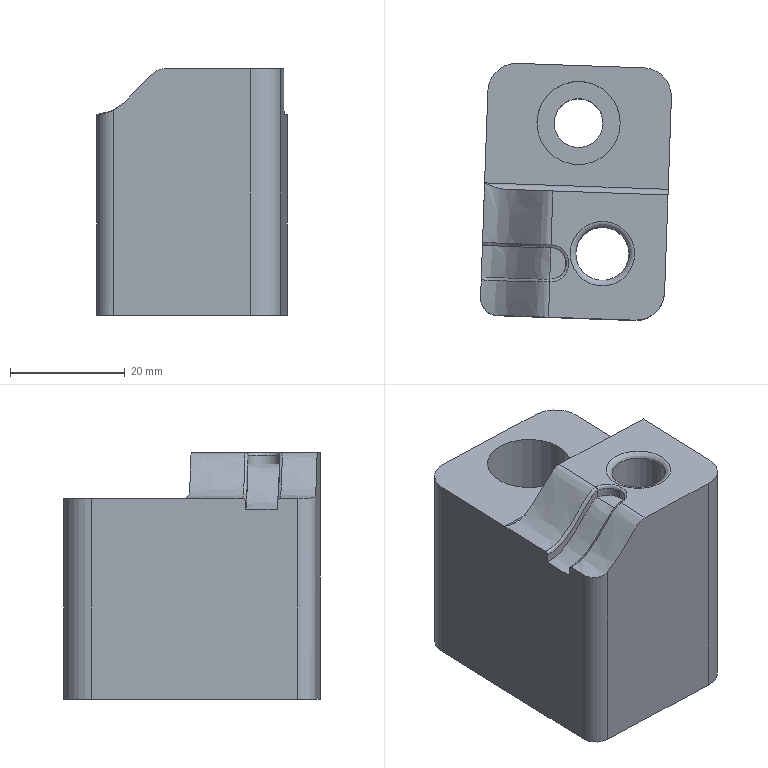Part | NX | features DIE-58 2 | 1 solid | 31 faces | box 33.242 x 44.747 x 43 mm | volume 45917 mm3 | plane 11 | spline 10 | cylinder 9 | torus 1 | commonest cylinder face diameters 10 x3 2 x1 6 x1 8.5 x1 9.27 x1 14 x1